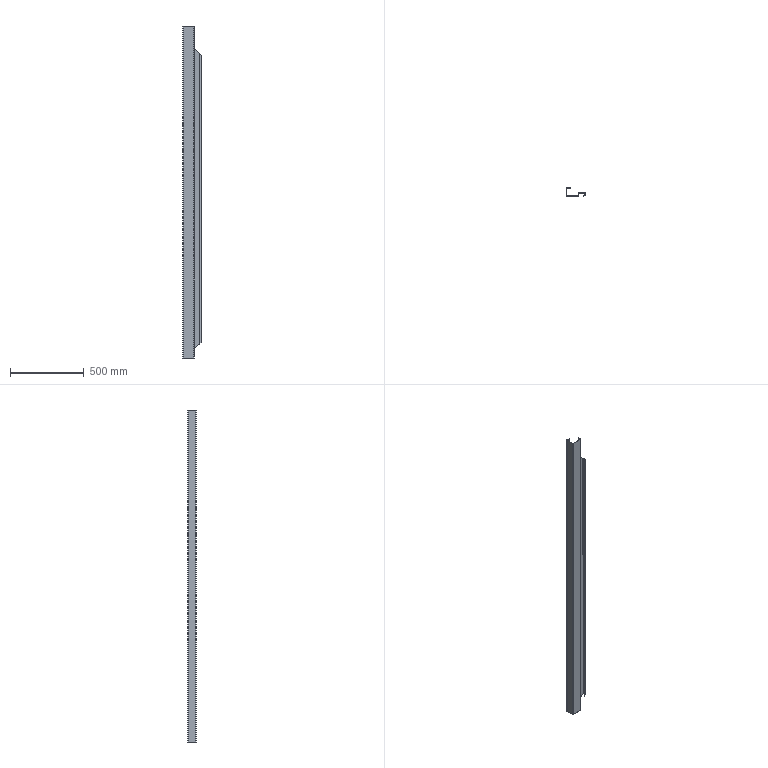Part | STEP file | 750038400 | 1 solid | 32 faces | box 127 x 60 x 2253 mm | volume 1105749 mm3 | plane 20 | cylinder 12 | commonest cylinder face diameters 4 x6 8 x6
STEP:
#1=CARTESIAN_POINT('',(4.,0.,0.));
#2=VERTEX_POINT('',#1);
#3=CARTESIAN_POINT('',(4.,0.,2252.5));
#4=VERTEX_POINT('',#3);
#5=CARTESIAN_POINT('',(4.,0.,0.));
#6=DIRECTION('',(0.,0.,1.));
#7=VECTOR('',#6,1000.);
#8=LINE('',#5,#7);
#9=EDGE_CURVE('',#2,#4,#8,.T.);
#10=ORIENTED_EDGE('',*,*,#9,.F.);
#11=CARTESIAN_POINT('',(76.,0.,0.));
#12=VERTEX_POINT('',#11);
#13=CARTESIAN_POINT('',(80.,0.,0.));
#14=DIRECTION('',(-1.,0.,0.));
#15=VECTOR('',#14,1000.);
#16=LINE('',#13,#15);
#17=EDGE_CURVE('',#12,#2,#16,.T.);
#18=ORIENTED_EDGE('',*,*,#17,.F.);
#19=CARTESIAN_POINT('',(76.,0.,2252.5));
#20=VERTEX_POINT('',#19);
#21=CARTESIAN_POINT('',(76.,0.,0.));
#22=DIRECTION('',(0.,0.,-1.));
#23=VECTOR('',#22,1000.);
#24=LINE('',#21,#23);
#25=EDGE_CURVE('',#20,#12,#24,.T.);
#26=ORIENTED_EDGE('',*,*,#25,.F.);
#27=CARTESIAN_POINT('',(80.,0.,2252.5));
#28=DIRECTION('',(1.,0.,0.));
#29=VECTOR('',#28,1000.);
#30=LINE('',#27,#29);
#31=EDGE_CURVE('',#4,#20,#30,.T.);
#32=ORIENTED_EDGE('',*,*,#31,.F.);
#33=EDGE_LOOP('',(#10,#18,#26,#32));
#34=FACE_OUTER_BOUND('',#33,.T.);
#35=CARTESIAN_POINT('',(80.,0.,0.));
#36=DIRECTION('',(0.,1.,0.));
#37=DIRECTION('',(0.,0.,1.));
#38=AXIS2_PLACEMENT_3D('',#35,#36,#37);
#39=PLANE('',#38);
#40=ADVANCED_FACE('',(#34),#39,.F.);
#41=ORIENTED_EDGE('',*,*,#31,.T.);
#42=CARTESIAN_POINT('',(80.,4.,2252.5));
#43=VERTEX_POINT('',#42);
#44=CARTESIAN_POINT('',(76.,4.,2252.5));
#45=DIRECTION('',(0.,0.,1.));
#46=DIRECTION('',(1.,0.,0.));
#47=AXIS2_PLACEMENT_3D('',#44,#45,#46);
#48=CIRCLE('',#47,4.);
#49=EDGE_CURVE('',#20,#43,#48,.T.);
#50=ORIENTED_EDGE('',*,*,#49,.T.);
#51=CARTESIAN_POINT('',(80.,26.464,2252.5));
#52=VERTEX_POINT('',#51);
#53=CARTESIAN_POINT('',(80.,10.535,2252.5));
#54=DIRECTION('',(0.,1.,0.));
#55=VECTOR('',#54,1000.);
#56=LINE('',#53,#55);
#57=EDGE_CURVE('',#43,#52,#56,.T.);
#58=ORIENTED_EDGE('',*,*,#57,.T.);
#59=CARTESIAN_POINT('',(78.,23.,2252.5));
#60=VERTEX_POINT('',#59);
#61=CARTESIAN_POINT('',(82.,23.,2252.5));
#62=DIRECTION('',(0.,0.,1.));
#63=DIRECTION('',(1.,0.,0.));
#64=AXIS2_PLACEMENT_3D('',#61,#62,#63);
#65=CIRCLE('',#64,4.);
#66=EDGE_CURVE('',#52,#60,#65,.T.);
#67=ORIENTED_EDGE('',*,*,#66,.T.);
#68=CARTESIAN_POINT('',(78.,4.,2252.5));
#69=VERTEX_POINT('',#68);
#70=CARTESIAN_POINT('',(78.,10.535,2252.5));
#71=DIRECTION('',(0.,-1.,0.));
#72=VECTOR('',#71,1000.);
#73=LINE('',#70,#72);
#74=EDGE_CURVE('',#60,#69,#73,.T.);
#75=ORIENTED_EDGE('',*,*,#74,.T.);
#76=CARTESIAN_POINT('',(76.,2.,2252.5));
#77=VERTEX_POINT('',#76);
#78=CARTESIAN_POINT('',(76.,4.,2252.5));
#79=DIRECTION('',(0.,0.,-1.));
#80=DIRECTION('',(1.,0.,0.));
#81=AXIS2_PLACEMENT_3D('',#78,#79,#80);
#82=CIRCLE('',#81,2.);
#83=EDGE_CURVE('',#69,#77,#82,.T.);
#84=ORIENTED_EDGE('',*,*,#83,.T.);
#85=CARTESIAN_POINT('',(4.,2.,2252.5));
#86=VERTEX_POINT('',#85);
#87=CARTESIAN_POINT('',(123.,2.,2252.5));
#88=DIRECTION('',(-1.,0.,0.));
#89=VECTOR('',#88,1000.);
#90=LINE('',#87,#89);
#91=EDGE_CURVE('',#77,#86,#90,.T.);
#92=ORIENTED_EDGE('',*,*,#91,.T.);
#93=CARTESIAN_POINT('',(2.,4.,2252.5));
#94=VERTEX_POINT('',#93);
#95=CARTESIAN_POINT('',(4.,4.,2252.5));
#96=DIRECTION('',(0.,0.,-1.));
#97=DIRECTION('',(1.,0.,0.));
#98=AXIS2_PLACEMENT_3D('',#95,#96,#97);
#99=CIRCLE('',#98,2.);
#100=EDGE_CURVE('',#86,#94,#99,.T.);
#101=ORIENTED_EDGE('',*,*,#100,.T.);
#102=CARTESIAN_POINT('',(2.,56.,2252.5));
#103=VERTEX_POINT('',#102);
#104=CARTESIAN_POINT('',(2.,10.535,2252.5));
#105=DIRECTION('',(0.,1.,0.));
#106=VECTOR('',#105,1000.);
#107=LINE('',#104,#106);
#108=EDGE_CURVE('',#94,#103,#107,.T.);
#109=ORIENTED_EDGE('',*,*,#108,.T.);
#110=CARTESIAN_POINT('',(4.,58.,2252.5));
#111=VERTEX_POINT('',#110);
#112=CARTESIAN_POINT('',(4.,56.,2252.5));
#113=DIRECTION('',(0.,0.,-1.));
#114=DIRECTION('',(1.,0.,0.));
#115=AXIS2_PLACEMENT_3D('',#112,#113,#114);
#116=CIRCLE('',#115,2.);
#117=EDGE_CURVE('',#103,#111,#116,.T.);
#118=ORIENTED_EDGE('',*,*,#117,.T.);
#119=CARTESIAN_POINT('',(25.,58.,2252.5));
#120=VERTEX_POINT('',#119);
#121=CARTESIAN_POINT('',(123.,58.,2252.5));
#122=DIRECTION('',(1.,0.,0.));
#123=VECTOR('',#122,1000.);
#124=LINE('',#121,#123);
#125=EDGE_CURVE('',#111,#120,#124,.T.);
#126=ORIENTED_EDGE('',*,*,#125,.T.);
#127=CARTESIAN_POINT('',(25.,60.,2252.5));
#128=VERTEX_POINT('',#127);
#129=CARTESIAN_POINT('',(25.,10.535,2252.5));
#130=DIRECTION('',(0.,1.,0.));
#131=VECTOR('',#130,1000.);
#132=LINE('',#129,#131);
#133=EDGE_CURVE('',#120,#128,#132,.T.);
#134=ORIENTED_EDGE('',*,*,#133,.T.);
#135=CARTESIAN_POINT('',(4.,60.,2252.5));
#136=VERTEX_POINT('',#135);
#137=CARTESIAN_POINT('',(123.,60.,2252.5));
#138=DIRECTION('',(-1.,0.,0.));
#139=VECTOR('',#138,1000.);
#140=LINE('',#137,#139);
#141=EDGE_CURVE('',#128,#136,#140,.T.);
#142=ORIENTED_EDGE('',*,*,#141,.T.);
#143=CARTESIAN_POINT('',(0.,56.,2252.5));
#144=VERTEX_POINT('',#143);
#145=CARTESIAN_POINT('',(4.,56.,2252.5));
#146=DIRECTION('',(0.,0.,1.));
#147=DIRECTION('',(1.,0.,0.));
#148=AXIS2_PLACEMENT_3D('',#145,#146,#147);
#149=CIRCLE('',#148,4.);
#150=EDGE_CURVE('',#136,#144,#149,.T.);
#151=ORIENTED_EDGE('',*,*,#150,.T.);
#152=CARTESIAN_POINT('',(0.,4.,2252.5));
#153=VERTEX_POINT('',#152);
#154=CARTESIAN_POINT('',(0.,10.535,2252.5));
#155=DIRECTION('',(0.,-1.,0.));
#156=VECTOR('',#155,1000.);
#157=LINE('',#154,#156);
#158=EDGE_CURVE('',#144,#153,#157,.T.);
#159=ORIENTED_EDGE('',*,*,#158,.T.);
#160=CARTESIAN_POINT('',(4.,4.,2252.5));
#161=DIRECTION('',(0.,0.,1.));
#162=DIRECTION('',(1.,0.,0.));
#163=AXIS2_PLACEMENT_3D('',#160,#161,#162);
#164=CIRCLE('',#163,4.);
#165=EDGE_CURVE('',#153,#4,#164,.T.);
#166=ORIENTED_EDGE('',*,*,#165,.T.);
#167=EDGE_LOOP('',(#41,#50,#58,#67,#75,#84,#92,#101,#109,#118,#126,#134,#142,#151,#159,#166));
#168=FACE_OUTER_BOUND('',#167,.T.);
#169=CARTESIAN_POINT('',(123.,10.535,2252.5));
#170=DIRECTION('',(0.,0.,1.));
#171=DIRECTION('',(1.,0.,0.));
#172=AXIS2_PLACEMENT_3D('',#169,#170,#171);
#173=PLANE('',#172);
#174=ADVANCED_FACE('',(#168),#173,.T.);
#175=CARTESIAN_POINT('',(0.,4.,0.));
#176=VERTEX_POINT('',#175);
#177=CARTESIAN_POINT('',(4.,4.,0.));
#178=DIRECTION('',(0.,0.,1.));
#179=DIRECTION('',(1.,0.,0.));
#180=AXIS2_PLACEMENT_3D('',#177,#178,#179);
#181=CIRCLE('',#180,4.);
#182=EDGE_CURVE('',#176,#2,#181,.T.);
#183=ORIENTED_EDGE('',*,*,#182,.T.);
#184=ORIENTED_EDGE('',*,*,#9,.T.);
#185=ORIENTED_EDGE('',*,*,#165,.F.);
#186=CARTESIAN_POINT('',(0.,4.,0.));
#187=DIRECTION('',(0.,0.,-1.));
#188=VECTOR('',#187,1000.);
#189=LINE('',#186,#188);
#190=EDGE_CURVE('',#153,#176,#189,.T.);
#191=ORIENTED_EDGE('',*,*,#190,.T.);
#192=EDGE_LOOP('',(#183,#184,#185,#191));
#193=FACE_OUTER_BOUND('',#192,.T.);
#194=CARTESIAN_POINT('',(4.,4.,0.));
#195=DIRECTION('',(0.,0.,1.));
#196=DIRECTION('',(1.,0.,0.));
#197=AXIS2_PLACEMENT_3D('',#194,#195,#196);
#198=CYLINDRICAL_SURFACE('',#197,4.);
#199=ADVANCED_FACE('',(#193),#198,.T.);
#200=CARTESIAN_POINT('',(76.,2.,0.));
#201=VERTEX_POINT('',#200);
#202=CARTESIAN_POINT('',(78.,4.,0.));
#203=VERTEX_POINT('',#202);
#204=CARTESIAN_POINT('',(76.,4.,0.));
#205=DIRECTION('',(0.,0.,1.));
#206=DIRECTION('',(1.,0.,0.));
#207=AXIS2_PLACEMENT_3D('',#204,#205,#206);
#208=CIRCLE('',#207,2.);
#209=EDGE_CURVE('',#201,#203,#208,.T.);
#210=ORIENTED_EDGE('',*,*,#209,.T.);
#211=CARTESIAN_POINT('',(78.,23.,0.));
#212=VERTEX_POINT('',#211);
#213=CARTESIAN_POINT('',(78.,6.153,0.));
#214=DIRECTION('',(0.,1.,0.));
#215=VECTOR('',#214,1000.);
#216=LINE('',#213,#215);
#217=EDGE_CURVE('',#203,#212,#216,.T.);
#218=ORIENTED_EDGE('',*,*,#217,.T.);
#219=CARTESIAN_POINT('',(80.,26.464,0.));
#220=VERTEX_POINT('',#219);
#221=CARTESIAN_POINT('',(82.,23.,0.));
#222=DIRECTION('',(0.,0.,-1.));
#223=DIRECTION('',(1.,0.,0.));
#224=AXIS2_PLACEMENT_3D('',#221,#222,#223);
#225=CIRCLE('',#224,4.);
#226=EDGE_CURVE('',#212,#220,#225,.T.);
#227=ORIENTED_EDGE('',*,*,#226,.T.);
#228=CARTESIAN_POINT('',(80.,4.,0.));
#229=VERTEX_POINT('',#228);
#230=CARTESIAN_POINT('',(80.,6.153,0.));
#231=DIRECTION('',(0.,-1.,0.));
#232=VECTOR('',#231,1000.);
#233=LINE('',#230,#232);
#234=EDGE_CURVE('',#220,#229,#233,.T.);
#235=ORIENTED_EDGE('',*,*,#234,.T.);
#236=CARTESIAN_POINT('',(76.,4.,0.));
#237=DIRECTION('',(0.,0.,-1.));
#238=DIRECTION('',(1.,0.,0.));
#239=AXIS2_PLACEMENT_3D('',#236,#237,#238);
#240=CIRCLE('',#239,4.);
#241=EDGE_CURVE('',#229,#12,#240,.T.);
#242=ORIENTED_EDGE('',*,*,#241,.T.);
#243=ORIENTED_EDGE('',*,*,#17,.T.);
#244=ORIENTED_EDGE('',*,*,#182,.F.);
#245=CARTESIAN_POINT('',(0.,56.,0.));
#246=VERTEX_POINT('',#245);
#247=CARTESIAN_POINT('',(0.,6.153,0.));
#248=DIRECTION('',(0.,1.,0.));
#249=VECTOR('',#248,1000.);
#250=LINE('',#247,#249);
#251=EDGE_CURVE('',#176,#246,#250,.T.);
#252=ORIENTED_EDGE('',*,*,#251,.T.);
#253=CARTESIAN_POINT('',(4.,60.,0.));
#254=VERTEX_POINT('',#253);
#255=CARTESIAN_POINT('',(4.,56.,0.));
#256=DIRECTION('',(0.,0.,-1.));
#257=DIRECTION('',(1.,0.,0.));
#258=AXIS2_PLACEMENT_3D('',#255,#256,#257);
#259=CIRCLE('',#258,4.);
#260=EDGE_CURVE('',#246,#254,#259,.T.);
#261=ORIENTED_EDGE('',*,*,#260,.T.);
#262=CARTESIAN_POINT('',(25.,60.,0.));
#263=VERTEX_POINT('',#262);
#264=CARTESIAN_POINT('',(114.375,60.,0.));
#265=DIRECTION('',(1.,0.,0.));
#266=VECTOR('',#265,1000.);
#267=LINE('',#264,#266);
#268=EDGE_CURVE('',#254,#263,#267,.T.);
#269=ORIENTED_EDGE('',*,*,#268,.T.);
#270=CARTESIAN_POINT('',(25.,58.,0.));
#271=VERTEX_POINT('',#270);
#272=CARTESIAN_POINT('',(25.,6.153,0.));
#273=DIRECTION('',(0.,-1.,0.));
#274=VECTOR('',#273,1000.);
#275=LINE('',#272,#274);
#276=EDGE_CURVE('',#263,#271,#275,.T.);
#277=ORIENTED_EDGE('',*,*,#276,.T.);
#278=CARTESIAN_POINT('',(4.,58.,0.));
#279=VERTEX_POINT('',#278);
#280=CARTESIAN_POINT('',(114.375,58.,0.));
#281=DIRECTION('',(-1.,0.,0.));
#282=VECTOR('',#281,1000.);
#283=LINE('',#280,#282);
#284=EDGE_CURVE('',#271,#279,#283,.T.);
#285=ORIENTED_EDGE('',*,*,#284,.T.);
#286=CARTESIAN_POINT('',(2.,56.,0.));
#287=VERTEX_POINT('',#286);
#288=CARTESIAN_POINT('',(4.,56.,0.));
#289=DIRECTION('',(0.,0.,1.));
#290=DIRECTION('',(1.,0.,0.));
#291=AXIS2_PLACEMENT_3D('',#288,#289,#290);
#292=CIRCLE('',#291,2.);
#293=EDGE_CURVE('',#279,#287,#292,.T.);
#294=ORIENTED_EDGE('',*,*,#293,.T.);
#295=CARTESIAN_POINT('',(2.,4.,0.));
#296=VERTEX_POINT('',#295);
#297=CARTESIAN_POINT('',(2.,6.153,0.));
#298=DIRECTION('',(0.,-1.,0.));
#299=VECTOR('',#298,1000.);
#300=LINE('',#297,#299);
#301=EDGE_CURVE('',#287,#296,#300,.T.);
#302=ORIENTED_EDGE('',*,*,#301,.T.);
#303=CARTESIAN_POINT('',(4.,2.,0.));
#304=VERTEX_POINT('',#303);
#305=CARTESIAN_POINT('',(4.,4.,0.));
#306=DIRECTION('',(0.,0.,1.));
#307=DIRECTION('',(1.,0.,0.));
#308=AXIS2_PLACEMENT_3D('',#305,#306,#307);
#309=CIRCLE('',#308,2.);
#310=EDGE_CURVE('',#296,#304,#309,.T.);
#311=ORIENTED_EDGE('',*,*,#310,.T.);
#312=CARTESIAN_POINT('',(114.375,2.,0.));
#313=DIRECTION('',(1.,0.,0.));
#314=VECTOR('',#313,1000.);
#315=LINE('',#312,#314);
#316=EDGE_CURVE('',#304,#201,#315,.T.);
#317=ORIENTED_EDGE('',*,*,#316,.T.);
#318=EDGE_LOOP('',(#210,#218,#227,#235,#242,#243,#244,#252,#261,#269,#277,#285,#294,#302,#311,#317));
#319=FACE_OUTER_BOUND('',#318,.T.);
#320=CARTESIAN_POINT('',(114.375,6.153,0.));
#321=DIRECTION('',(0.,0.,-1.));
#322=DIRECTION('',(-1.,0.,0.));
#323=AXIS2_PLACEMENT_3D('',#320,#321,#322);
#324=PLANE('',#323);
#325=ADVANCED_FACE('',(#319),#324,.T.);
#326=ORIENTED_EDGE('',*,*,#241,.F.);
#327=CARTESIAN_POINT('',(80.,4.,0.));
#328=DIRECTION('',(0.,0.,1.));
#329=VECTOR('',#328,1000.);
#330=LINE('',#327,#329);
#331=EDGE_CURVE('',#229,#43,#330,.T.);
#332=ORIENTED_EDGE('',*,*,#331,.T.);
#333=ORIENTED_EDGE('',*,*,#49,.F.);
#334=ORIENTED_EDGE('',*,*,#25,.T.);
#335=EDGE_LOOP('',(#326,#332,#333,#334));
#336=FACE_OUTER_BOUND('',#335,.T.);
#337=CARTESIAN_POINT('',(76.,4.,0.));
#338=DIRECTION('',(0.,0.,1.));
#339=DIRECTION('',(1.,0.,0.));
#340=AXIS2_PLACEMENT_3D('',#337,#338,#339);
#341=CYLINDRICAL_SURFACE('',#340,4.);
#342=ADVANCED_FACE('',(#336),#341,.T.);
#343=CARTESIAN_POINT('',(0.,56.,0.));
#344=DIRECTION('',(0.,0.,1.));
#345=VECTOR('',#344,1000.);
#346=LINE('',#343,#345);
#347=EDGE_CURVE('',#246,#144,#346,.T.);
#348=ORIENTED_EDGE('',*,*,#347,.F.);
#349=ORIENTED_EDGE('',*,*,#251,.F.);
#350=ORIENTED_EDGE('',*,*,#190,.F.);
#351=ORIENTED_EDGE('',*,*,#158,.F.);
#352=EDGE_LOOP('',(#348,#349,#350,#351));
#353=FACE_OUTER_BOUND('',#352,.T.);
#354=CARTESIAN_POINT('',(0.,0.,0.));
#355=DIRECTION('',(1.,0.,0.));
#356=DIRECTION('',(0.,0.,-1.));
#357=AXIS2_PLACEMENT_3D('',#354,#355,#356);
#358=PLANE('',#357);
#359=ADVANCED_FACE('',(#353),#358,.F.);
#360=ORIENTED_EDGE('',*,*,#260,.F.);
#361=ORIENTED_EDGE('',*,*,#347,.T.);
#362=ORIENTED_EDGE('',*,*,#150,.F.);
#363=CARTESIAN_POINT('',(4.,60.,0.));
#364=DIRECTION('',(0.,0.,-1.));
#365=VECTOR('',#364,1000.);
#366=LINE('',#363,#365);
#367=EDGE_CURVE('',#136,#254,#366,.T.);
#368=ORIENTED_EDGE('',*,*,#367,.T.);
#369=EDGE_LOOP('',(#360,#361,#362,#368));
#370=FACE_OUTER_BOUND('',#369,.T.);
#371=CARTESIAN_POINT('',(4.,56.,0.));
#372=DIRECTION('',(0.,0.,1.));
#373=DIRECTION('',(1.,0.,0.));
#374=AXIS2_PLACEMENT_3D('',#371,#372,#373);
#375=CYLINDRICAL_SURFACE('',#374,4.);
#376=ADVANCED_FACE('',(#370),#375,.T.);
#377=CARTESIAN_POINT('',(25.,60.,0.));
#378=DIRECTION('',(0.,0.,1.));
#379=VECTOR('',#378,1000.);
#380=LINE('',#377,#379);
#381=EDGE_CURVE('',#263,#128,#380,.T.);
#382=ORIENTED_EDGE('',*,*,#381,.F.);
#383=ORIENTED_EDGE('',*,*,#268,.F.);
#384=ORIENTED_EDGE('',*,*,#367,.F.);
#385=ORIENTED_EDGE('',*,*,#141,.F.);
#386=EDGE_LOOP('',(#382,#383,#384,#385));
#387=FACE_OUTER_BOUND('',#386,.T.);
#388=CARTESIAN_POINT('',(0.,60.,0.));
#389=DIRECTION('',(0.,-1.,0.));
#390=DIRECTION('',(0.,0.,-1.));
#391=AXIS2_PLACEMENT_3D('',#388,#389,#390);
#392=PLANE('',#391);
#393=ADVANCED_FACE('',(#387),#392,.F.);
#394=ORIENTED_EDGE('',*,*,#276,.F.);
#395=ORIENTED_EDGE('',*,*,#381,.T.);
#396=ORIENTED_EDGE('',*,*,#133,.F.);
#397=CARTESIAN_POINT('',(25.,58.,0.));
#398=DIRECTION('',(0.,0.,-1.));
#399=VECTOR('',#398,1000.);
#400=LINE('',#397,#399);
#401=EDGE_CURVE('',#120,#271,#400,.T.);
#402=ORIENTED_EDGE('',*,*,#401,.T.);
#403=EDGE_LOOP('',(#394,#395,#396,#402));
#404=FACE_OUTER_BOUND('',#403,.T.);
#405=CARTESIAN_POINT('',(25.,60.,0.));
#406=DIRECTION('',(1.,0.,0.));
#407=DIRECTION('',(0.,0.,-1.));
#408=AXIS2_PLACEMENT_3D('',#405,#406,#407);
#409=PLANE('',#408);
#410=ADVANCED_FACE('',(#404),#409,.T.);
#411=ORIENTED_EDGE('',*,*,#284,.F.);
#412=ORIENTED_EDGE('',*,*,#401,.F.);
#413=ORIENTED_EDGE('',*,*,#125,.F.);
#414=CARTESIAN_POINT('',(4.,58.,0.));
#415=DIRECTION('',(0.,0.,-1.));
#416=VECTOR('',#415,1000.);
#417=LINE('',#414,#416);
#418=EDGE_CURVE('',#111,#279,#417,.T.);
#419=ORIENTED_EDGE('',*,*,#418,.T.);
#420=EDGE_LOOP('',(#411,#412,#413,#419));
#421=FACE_OUTER_BOUND('',#420,.T.);
#422=CARTESIAN_POINT('',(0.,58.,0.));
#423=DIRECTION('',(0.,-1.,0.));
#424=DIRECTION('',(0.,0.,-1.));
#425=AXIS2_PLACEMENT_3D('',#422,#423,#424);
#426=PLANE('',#425);
#427=ADVANCED_FACE('',(#421),#426,.T.);
#428=CARTESIAN_POINT('',(2.,56.,0.));
#429=DIRECTION('',(0.,0.,1.));
#430=VECTOR('',#429,1000.);
#431=LINE('',#428,#430);
#432=EDGE_CURVE('',#287,#103,#431,.T.);
#433=ORIENTED_EDGE('',*,*,#432,.F.);
#434=ORIENTED_EDGE('',*,*,#293,.F.);
#435=ORIENTED_EDGE('',*,*,#418,.F.);
#436=ORIENTED_EDGE('',*,*,#117,.F.);
#437=EDGE_LOOP('',(#433,#434,#435,#436));
#438=FACE_OUTER_BOUND('',#437,.T.);
#439=CARTESIAN_POINT('',(4.,56.,0.));
#440=DIRECTION('',(0.,0.,1.));
#441=DIRECTION('',(1.,0.,0.));
#442=AXIS2_PLACEMENT_3D('',#439,#440,#441);
#443=CYLINDRICAL_SURFACE('',#442,2.);
#444=ADVANCED_FACE('',(#438),#443,.F.);
#445=ORIENTED_EDGE('',*,*,#301,.F.);
#446=ORIENTED_EDGE('',*,*,#432,.T.);
#447=ORIENTED_EDGE('',*,*,#108,.F.);
#448=CARTESIAN_POINT('',(2.,4.,0.));
#449=DIRECTION('',(0.,0.,-1.));
#450=VECTOR('',#449,1000.);
#451=LINE('',#448,#450);
#452=EDGE_CURVE('',#94,#296,#451,.T.);
#453=ORIENTED_EDGE('',*,*,#452,.T.);
#454=EDGE_LOOP('',(#445,#446,#447,#453));
#455=FACE_OUTER_BOUND('',#454,.T.);
#456=CARTESIAN_POINT('',(2.,0.,0.));
#457=DIRECTION('',(1.,0.,0.));
#458=DIRECTION('',(0.,0.,-1.));
#459=AXIS2_PLACEMENT_3D('',#456,#457,#458);
#460=PLANE('',#459);
#461=ADVANCED_FACE('',(#455),#460,.T.);
#462=CARTESIAN_POINT('',(4.,2.,0.));
#463=DIRECTION('',(0.,0.,1.));
#464=VECTOR('',#463,1000.);
#465=LINE('',#462,#464);
#466=EDGE_CURVE('',#304,#86,#465,.T.);
#467=ORIENTED_EDGE('',*,*,#466,.F.);
#468=ORIENTED_EDGE('',*,*,#310,.F.);
#469=ORIENTED_EDGE('',*,*,#452,.F.);
#470=ORIENTED_EDGE('',*,*,#100,.F.);
#471=EDGE_LOOP('',(#467,#468,#469,#470));
#472=FACE_OUTER_BOUND('',#471,.T.);
#473=CARTESIAN_POINT('',(4.,4.,0.));
#474=DIRECTION('',(0.,0.,1.));
#475=DIRECTION('',(1.,0.,0.));
#476=AXIS2_PLACEMENT_3D('',#473,#474,#475);
#477=CYLINDRICAL_SURFACE('',#476,2.);
#478=ADVANCED_FACE('',(#472),#477,.F.);
#479=ORIENTED_EDGE('',*,*,#316,.F.);
#480=ORIENTED_EDGE('',*,*,#466,.T.);
#481=ORIENTED_EDGE('',*,*,#91,.F.);
#482=CARTESIAN_POINT('',(76.,2.,0.));
#483=DIRECTION('',(0.,0.,-1.));
#484=VECTOR('',#483,1000.);
#485=LINE('',#482,#484);
#486=EDGE_CURVE('',#77,#201,#485,.T.);
#487=ORIENTED_EDGE('',*,*,#486,.T.);
#488=EDGE_LOOP('',(#479,#480,#481,#487));
#489=FACE_OUTER_BOUND('',#488,.T.);
#490=CARTESIAN_POINT('',(80.,2.,0.));
#491=DIRECTION('',(0.,1.,0.));
#492=DIRECTION('',(0.,0.,1.));
#493=AXIS2_PLACEMENT_3D('',#490,#491,#492);
#494=PLANE('',#493);
#495=ADVANCED_FACE('',(#489),#494,.T.);
#496=CARTESIAN_POINT('',(78.,4.,0.));
#497=DIRECTION('',(0.,0.,1.));
#498=VECTOR('',#497,1000.);
#499=LINE('',#496,#498);
#500=EDGE_CURVE('',#203,#69,#499,.T.);
#501=ORIENTED_EDGE('',*,*,#500,.F.);
#502=ORIENTED_EDGE('',*,*,#209,.F.);
#503=ORIENTED_EDGE('',*,*,#486,.F.);
#504=ORIENTED_EDGE('',*,*,#83,.F.);
#505=EDGE_LOOP('',(#501,#502,#503,#504));
#506=FACE_OUTER_BOUND('',#505,.T.);
#507=CARTESIAN_POINT('',(76.,4.,0.));
#508=DIRECTION('',(0.,0.,1.));
#509=DIRECTION('',(1.,0.,0.));
#510=AXIS2_PLACEMENT_3D('',#507,#508,#509);
#511=CYLINDRICAL_SURFACE('',#510,2.);
#512=ADVANCED_FACE('',(#506),#511,.F.);
#513=ORIENTED_EDGE('',*,*,#217,.F.);
#514=ORIENTED_EDGE('',*,*,#500,.T.);
#515=ORIENTED_EDGE('',*,*,#74,.F.);
#516=CARTESIAN_POINT('',(78.,23.,0.));
#517=DIRECTION('',(0.,0.,-1.));
#518=VECTOR('',#517,1000.);
#519=LINE('',#516,#518);
#520=EDGE_CURVE('',#60,#212,#519,.T.);
#521=ORIENTED_EDGE('',*,*,#520,.T.);
#522=EDGE_LOOP('',(#513,#514,#515,#521));
#523=FACE_OUTER_BOUND('',#522,.T.);
#524=CARTESIAN_POINT('',(78.,25.,0.));
#525=DIRECTION('',(-1.,0.,0.));
#526=DIRECTION('',(0.,-1.,0.));
#527=AXIS2_PLACEMENT_3D('',#524,#525,#526);
#528=PLANE('',#527);
#529=ADVANCED_FACE('',(#523),#528,.T.);
#530=CARTESIAN_POINT('',(82.,27.,2098.));
#531=VERTEX_POINT('',#530);
#532=CARTESIAN_POINT('',(82.,27.,62.));
#533=VERTEX_POINT('',#532);
#534=CARTESIAN_POINT('',(82.,27.,0.));
#535=DIRECTION('',(0.,0.,-1.));
#536=VECTOR('',#535,1000.);
#537=LINE('',#534,#536);
#538=EDGE_CURVE('',#531,#533,#537,.T.);
#539=ORIENTED_EDGE('',*,*,#538,.T.);
#540=CARTESIAN_POINT('',(80.,26.464,60.));
#541=VERTEX_POINT('',#540);
#542=CARTESIAN_POINT('',(82.,27.,62.));
#543=CARTESIAN_POINT('',(81.294,27.,61.294));
#544=CARTESIAN_POINT('',(80.612,26.817,60.612));
#545=CARTESIAN_POINT('',(80.,26.464,60.));
#546=(BOUNDED_CURVE()B_SPLINE_CURVE(3,(#542,#543,#544,#545),.UNSPECIFIED.,.F.,.F.)B_SPLINE_CURVE_WITH_KNOTS((4,4),(1.571,2.094),.UNSPECIFIED.)CURVE()GEOMETRIC_REPRESENTATION_ITEM()RATIONAL_B_SPLINE_CURVE((1.,0.9773,0.9773,1.))REPRESENTATION_ITEM(''));
#547=EDGE_CURVE('',#533,#541,#546,.T.);
#548=ORIENTED_EDGE('',*,*,#547,.T.);
#549=CARTESIAN_POINT('',(80.,26.464,0.));
#550=DIRECTION('',(0.,0.,-1.));
#551=VECTOR('',#550,1000.);
#552=LINE('',#549,#551);
#553=EDGE_CURVE('',#541,#220,#552,.T.);
#554=ORIENTED_EDGE('',*,*,#553,.T.);
#555=ORIENTED_EDGE('',*,*,#226,.F.);
#556=ORIENTED_EDGE('',*,*,#520,.F.);
#557=ORIENTED_EDGE('',*,*,#66,.F.);
#558=CARTESIAN_POINT('',(80.,26.464,2100.));
#559=VERTEX_POINT('',#558);
#560=CARTESIAN_POINT('',(80.,26.464,0.));
#561=DIRECTION('',(0.,0.,-1.));
#562=VECTOR('',#561,1000.);
#563=LINE('',#560,#562);
#564=EDGE_CURVE('',#52,#559,#563,.T.);
#565=ORIENTED_EDGE('',*,*,#564,.T.);
#566=CARTESIAN_POINT('',(80.,26.464,2100.));
#567=CARTESIAN_POINT('',(80.612,26.817,2099.388));
#568=CARTESIAN_POINT('',(81.294,27.,2098.706));
#569=CARTESIAN_POINT('',(82.,27.,2098.));
#570=(BOUNDED_CURVE()B_SPLINE_CURVE(3,(#566,#567,#568,#569),.UNSPECIFIED.,.F.,.F.)B_SPLINE_CURVE_WITH_KNOTS((4,4),(1.047,1.571),.UNSPECIFIED.)CURVE()GEOMETRIC_REPRESENTATION_ITEM()RATIONAL_B_SPLINE_CURVE((1.,0.9773,0.9773,1.))REPRESENTATION_ITEM(''));
#571=EDGE_CURVE('',#559,#531,#570,.T.);
#572=ORIENTED_EDGE('',*,*,#571,.T.);
#573=EDGE_LOOP('',(#539,#548,#554,#555,#556,#557,#565,#572));
#574=FACE_OUTER_BOUND('',#573,.T.);
#575=CARTESIAN_POINT('',(82.,23.,0.));
#576=DIRECTION('',(0.,0.,1.));
#577=DIRECTION('',(1.,0.,0.));
#578=AXIS2_PLACEMENT_3D('',#575,#576,#577);
#579=CYLINDRICAL_SURFACE('',#578,4.);
#580=ADVANCED_FACE('',(#574),#579,.T.);
#581=ORIENTED_EDGE('',*,*,#553,.F.);
#582=CARTESIAN_POINT('',(80.,23.,60.));
#583=VERTEX_POINT('',#582);
#584=CARTESIAN_POINT('',(80.,25.,60.));
#585=DIRECTION('',(0.,1.,0.));
#586=VECTOR('',#585,1000.);
#587=LINE('',#584,#586);
#588=EDGE_CURVE('',#583,#541,#587,.T.);
#589=ORIENTED_EDGE('',*,*,#588,.F.);
#590=CARTESIAN_POINT('',(80.,23.,2100.));
#591=VERTEX_POINT('',#590);
#592=CARTESIAN_POINT('',(80.,23.,0.));
#593=DIRECTION('',(0.,0.,-1.));
#594=VECTOR('',#593,1000.);
#595=LINE('',#592,#594);
#596=EDGE_CURVE('',#591,#583,#595,.T.);
#597=ORIENTED_EDGE('',*,*,#596,.F.);
#598=CARTESIAN_POINT('',(80.,25.,2100.));
#599=DIRECTION('',(0.,-1.,0.));
#600=VECTOR('',#599,1000.);
#601=LINE('',#598,#600);
#602=EDGE_CURVE('',#559,#591,#601,.T.);
#603=ORIENTED_EDGE('',*,*,#602,.F.);
#604=ORIENTED_EDGE('',*,*,#564,.F.);
#605=ORIENTED_EDGE('',*,*,#57,.F.);
#606=ORIENTED_EDGE('',*,*,#331,.F.);
#607=ORIENTED_EDGE('',*,*,#234,.F.);
#608=EDGE_LOOP('',(#581,#589,#597,#603,#604,#605,#606,#607));
#609=FACE_OUTER_BOUND('',#608,.T.);
#610=CARTESIAN_POINT('',(80.,25.,0.));
#611=DIRECTION('',(-1.,0.,0.));
#612=DIRECTION('',(0.,-1.,0.));
#613=AXIS2_PLACEMENT_3D('',#610,#611,#612);
#614=PLANE('',#613);
#615=ADVANCED_FACE('',(#609),#614,.F.);
#616=ORIENTED_EDGE('',*,*,#547,.F.);
#617=CARTESIAN_POINT('',(123.,27.,103.));
#618=VERTEX_POINT('',#617);
#619=CARTESIAN_POINT('',(127.376,27.,107.376));
#620=DIRECTION('',(-0.7071,0.,-0.7071));
#621=VECTOR('',#620,1000.);
#622=LINE('',#619,#621);
#623=EDGE_CURVE('',#618,#533,#622,.T.);
#624=ORIENTED_EDGE('',*,*,#623,.F.);
#625=CARTESIAN_POINT('',(127.,23.,107.));
#626=VERTEX_POINT('',#625);
#627=CARTESIAN_POINT('',(127.,23.,107.));
#628=CARTESIAN_POINT('',(127.,25.343,107.));
#629=CARTESIAN_POINT('',(125.343,27.,105.343));
#630=CARTESIAN_POINT('',(123.,27.,103.));
#631=(BOUNDED_CURVE()B_SPLINE_CURVE(3,(#627,#628,#629,#630),.UNSPECIFIED.,.F.,.F.)B_SPLINE_CURVE_WITH_KNOTS((4,4),(0.,1.571),.UNSPECIFIED.)CURVE()GEOMETRIC_REPRESENTATION_ITEM()RATIONAL_B_SPLINE_CURVE((1.,0.8047,0.8047,1.))REPRESENTATION_ITEM(''));
#632=EDGE_CURVE('',#626,#618,#631,.T.);
#633=ORIENTED_EDGE('',*,*,#632,.F.);
#634=CARTESIAN_POINT('',(127.,10.535,107.));
#635=VERTEX_POINT('',#634);
#636=CARTESIAN_POINT('',(127.,66.,107.));
#637=DIRECTION('',(0.,1.,0.));
#638=VECTOR('',#637,1000.);
#639=LINE('',#636,#638);
#640=EDGE_CURVE('',#635,#626,#639,.T.);
#641=ORIENTED_EDGE('',*,*,#640,.F.);
#642=CARTESIAN_POINT('',(124.035,6.671,104.035));
#643=VERTEX_POINT('',#642);
#644=CARTESIAN_POINT('',(124.035,6.671,104.035));
#645=CARTESIAN_POINT('',(125.854,7.158,105.854));
#646=CARTESIAN_POINT('',(127.,8.652,107.));
#647=CARTESIAN_POINT('',(127.,10.535,107.));
#648=(BOUNDED_CURVE()B_SPLINE_CURVE(3,(#644,#645,#646,#647),.UNSPECIFIED.,.F.,.F.)B_SPLINE_CURVE_WITH_KNOTS((4,4),(4.974,6.283),.UNSPECIFIED.)CURVE()GEOMETRIC_REPRESENTATION_ITEM()RATIONAL_B_SPLINE_CURVE((1.,0.8622,0.8622,1.))REPRESENTATION_ITEM(''));
#649=EDGE_CURVE('',#643,#635,#648,.T.);
#650=ORIENTED_EDGE('',*,*,#649,.F.);
#651=CARTESIAN_POINT('',(114.892,4.221,94.892));
#652=VERTEX_POINT('',#651);
#653=CARTESIAN_POINT('',(114.892,4.221,94.892));
#654=DIRECTION('',(0.6947,0.1862,0.6947));
#655=VECTOR('',#654,1000.);
#656=LINE('',#653,#655);
#657=EDGE_CURVE('',#652,#643,#656,.T.);
#658=ORIENTED_EDGE('',*,*,#657,.F.);
#659=CARTESIAN_POINT('',(114.375,6.153,94.375));
#660=VERTEX_POINT('',#659);
#661=CARTESIAN_POINT('',(114.375,6.153,94.375));
#662=DIRECTION('',(0.2506,-0.9351,0.2506));
#663=VECTOR('',#662,1000.);
#664=LINE('',#661,#663);
#665=EDGE_CURVE('',#660,#652,#664,.T.);
#666=ORIENTED_EDGE('',*,*,#665,.F.);
#667=CARTESIAN_POINT('',(123.518,8.603,103.518));
#668=VERTEX_POINT('',#667);
#669=CARTESIAN_POINT('',(123.518,8.603,103.518));
#670=DIRECTION('',(-0.6947,-0.1862,-0.6947));
#671=VECTOR('',#670,1000.);
#672=LINE('',#669,#671);
#673=EDGE_CURVE('',#668,#660,#672,.T.);
#674=ORIENTED_EDGE('',*,*,#673,.F.);
#675=CARTESIAN_POINT('',(125.,10.535,105.));
#676=VERTEX_POINT('',#675);
#677=CARTESIAN_POINT('',(125.,10.535,105.));
#678=CARTESIAN_POINT('',(125.,9.593,105.));
#679=CARTESIAN_POINT('',(124.427,8.846,104.427));
#680=CARTESIAN_POINT('',(123.518,8.603,103.518));
#681=(BOUNDED_CURVE()B_SPLINE_CURVE(3,(#677,#678,#679,#680),.UNSPECIFIED.,.F.,.F.)B_SPLINE_CURVE_WITH_KNOTS((4,4),(0.,1.309),.UNSPECIFIED.)CURVE()GEOMETRIC_REPRESENTATION_ITEM()RATIONAL_B_SPLINE_CURVE((1.,0.8622,0.8622,1.))REPRESENTATION_ITEM(''));
#682=EDGE_CURVE('',#676,#668,#681,.T.);
#683=ORIENTED_EDGE('',*,*,#682,.F.);
#684=CARTESIAN_POINT('',(125.,23.,105.));
#685=VERTEX_POINT('',#684);
#686=CARTESIAN_POINT('',(125.,66.,105.));
#687=DIRECTION('',(0.,-1.,0.));
#688=VECTOR('',#687,1000.);
#689=LINE('',#686,#688);
#690=EDGE_CURVE('',#685,#676,#689,.T.);
#691=ORIENTED_EDGE('',*,*,#690,.F.);
#692=CARTESIAN_POINT('',(123.,25.,103.));
#693=VERTEX_POINT('',#692);
#694=CARTESIAN_POINT('',(123.,25.,103.));
#695=CARTESIAN_POINT('',(124.172,25.,104.172));
#696=CARTESIAN_POINT('',(125.,24.172,105.));
#697=CARTESIAN_POINT('',(125.,23.,105.));
#698=(BOUNDED_CURVE()B_SPLINE_CURVE(3,(#694,#695,#696,#697),.UNSPECIFIED.,.F.,.F.)B_SPLINE_CURVE_WITH_KNOTS((4,4),(4.712,6.283),.UNSPECIFIED.)CURVE()GEOMETRIC_REPRESENTATION_ITEM()RATIONAL_B_SPLINE_CURVE((1.,0.8047,0.8047,1.))REPRESENTATION_ITEM(''));
#699=EDGE_CURVE('',#693,#685,#698,.T.);
#700=ORIENTED_EDGE('',*,*,#699,.F.);
#701=CARTESIAN_POINT('',(82.,25.,62.));
#702=VERTEX_POINT('',#701);
#703=CARTESIAN_POINT('',(127.376,25.,107.376));
#704=DIRECTION('',(0.7071,0.,0.7071));
#705=VECTOR('',#704,1000.);
#706=LINE('',#703,#705);
#707=EDGE_CURVE('',#702,#693,#706,.T.);
#708=ORIENTED_EDGE('',*,*,#707,.F.);
#709=CARTESIAN_POINT('',(80.,23.,60.));
#710=CARTESIAN_POINT('',(80.,24.172,60.));
#711=CARTESIAN_POINT('',(80.828,25.,60.828));
#712=CARTESIAN_POINT('',(82.,25.,62.));
#713=(BOUNDED_CURVE()B_SPLINE_CURVE(3,(#709,#710,#711,#712),.UNSPECIFIED.,.F.,.F.)B_SPLINE_CURVE_WITH_KNOTS((4,4),(3.142,4.712),.UNSPECIFIED.)CURVE()GEOMETRIC_REPRESENTATION_ITEM()RATIONAL_B_SPLINE_CURVE((1.,0.8047,0.8047,1.))REPRESENTATION_ITEM(''));
#714=EDGE_CURVE('',#583,#702,#713,.T.);
#715=ORIENTED_EDGE('',*,*,#714,.F.);
#716=ORIENTED_EDGE('',*,*,#588,.T.);
#717=EDGE_LOOP('',(#616,#624,#633,#641,#650,#658,#666,#674,#683,#691,#700,#708,#715,#716));
#718=FACE_OUTER_BOUND('',#717,.T.);
#719=CARTESIAN_POINT('',(127.376,66.,107.376));
#720=DIRECTION('',(-0.7071,0.,0.7071));
#721=DIRECTION('',(0.7071,0.,0.7071));
#722=AXIS2_PLACEMENT_3D('',#719,#720,#721);
#723=PLANE('',#722);
#724=ADVANCED_FACE('',(#718),#723,.F.);
#725=CARTESIAN_POINT('',(123.,27.,2057.));
#726=VERTEX_POINT('',#725);
#727=CARTESIAN_POINT('',(82.,27.,2098.));
#728=DIRECTION('',(0.7071,0.,-0.7071));
#729=VECTOR('',#728,1000.);
#730=LINE('',#727,#729);
#731=EDGE_CURVE('',#531,#726,#730,.T.);
#732=ORIENTED_EDGE('',*,*,#731,.T.);
#733=CARTESIAN_POINT('',(123.,27.,0.));
#734=DIRECTION('',(0.,0.,-1.));
#735=VECTOR('',#734,1000.);
#736=LINE('',#733,#735);
#737=EDGE_CURVE('',#726,#618,#736,.T.);
#738=ORIENTED_EDGE('',*,*,#737,.T.);
#739=ORIENTED_EDGE('',*,*,#623,.T.);
#740=ORIENTED_EDGE('',*,*,#538,.F.);
#741=EDGE_LOOP('',(#732,#738,#739,#740));
#742=FACE_OUTER_BOUND('',#741,.T.);
#743=CARTESIAN_POINT('',(125.,27.,0.));
#744=DIRECTION('',(0.,1.,0.));
#745=DIRECTION('',(0.,0.,1.));
#746=AXIS2_PLACEMENT_3D('',#743,#744,#745);
#747=PLANE('',#746);
#748=ADVANCED_FACE('',(#742),#747,.T.);
#749=CARTESIAN_POINT('',(125.,23.,2055.));
#750=VERTEX_POINT('',#749);
#751=CARTESIAN_POINT('',(123.,25.,2057.));
#752=VERTEX_POINT('',#751);
#753=CARTESIAN_POINT('',(125.,23.,2055.));
#754=CARTESIAN_POINT('',(125.,24.172,2055.));
#755=CARTESIAN_POINT('',(124.172,25.,2055.828));
#756=CARTESIAN_POINT('',(123.,25.,2057.));
#757=(BOUNDED_CURVE()B_SPLINE_CURVE(3,(#753,#754,#755,#756),.UNSPECIFIED.,.F.,.T.)B_SPLINE_CURVE_WITH_KNOTS((4,4),(3.142,4.712),.UNSPECIFIED.)CURVE()GEOMETRIC_REPRESENTATION_ITEM()RATIONAL_B_SPLINE_CURVE((1.,0.8047,0.8047,1.))REPRESENTATION_ITEM(''));
#758=EDGE_CURVE('',#750,#752,#757,.T.);
#759=ORIENTED_EDGE('',*,*,#758,.F.);
#760=CARTESIAN_POINT('',(125.,10.535,2055.));
#761=VERTEX_POINT('',#760);
#762=CARTESIAN_POINT('',(125.,66.,2055.));
#763=DIRECTION('',(0.,1.,0.));
#764=VECTOR('',#763,1000.);
#765=LINE('',#762,#764);
#766=EDGE_CURVE('',#761,#750,#765,.T.);
#767=ORIENTED_EDGE('',*,*,#766,.F.);
#768=CARTESIAN_POINT('',(123.518,8.603,2056.482));
#769=VERTEX_POINT('',#768);
#770=CARTESIAN_POINT('',(123.518,8.603,2056.482));
#771=CARTESIAN_POINT('',(124.427,8.846,2055.573));
#772=CARTESIAN_POINT('',(125.,9.593,2055.));
#773=CARTESIAN_POINT('',(125.,10.535,2055.));
#774=(BOUNDED_CURVE()B_SPLINE_CURVE(3,(#770,#771,#772,#773),.UNSPECIFIED.,.F.,.F.)B_SPLINE_CURVE_WITH_KNOTS((4,4),(1.833,3.142),.UNSPECIFIED.)CURVE()GEOMETRIC_REPRESENTATION_ITEM()RATIONAL_B_SPLINE_CURVE((1.,0.8622,0.8622,1.))REPRESENTATION_ITEM(''));
#775=EDGE_CURVE('',#769,#761,#774,.T.);
#776=ORIENTED_EDGE('',*,*,#775,.F.);
#777=CARTESIAN_POINT('',(114.375,6.153,2065.625));
#778=VERTEX_POINT('',#777);
#779=CARTESIAN_POINT('',(114.375,6.153,2065.625));
#780=DIRECTION('',(0.6947,0.1862,-0.6947));
#781=VECTOR('',#780,1000.);
#782=LINE('',#779,#781);
#783=EDGE_CURVE('',#778,#769,#782,.T.);
#784=ORIENTED_EDGE('',*,*,#783,.F.);
#785=CARTESIAN_POINT('',(114.892,4.221,2065.108));
#786=VERTEX_POINT('',#785);
#787=CARTESIAN_POINT('',(114.892,4.221,2065.108));
#788=DIRECTION('',(-0.2506,0.9351,0.2506));
#789=VECTOR('',#788,1000.);
#790=LINE('',#787,#789);
#791=EDGE_CURVE('',#786,#778,#790,.T.);
#792=ORIENTED_EDGE('',*,*,#791,.F.);
#793=CARTESIAN_POINT('',(124.035,6.671,2055.965));
#794=VERTEX_POINT('',#793);
#795=CARTESIAN_POINT('',(124.035,6.671,2055.965));
#796=DIRECTION('',(-0.6947,-0.1862,0.6947));
#797=VECTOR('',#796,1000.);
#798=LINE('',#795,#797);
#799=EDGE_CURVE('',#794,#786,#798,.T.);
#800=ORIENTED_EDGE('',*,*,#799,.F.);
#801=CARTESIAN_POINT('',(127.,10.535,2053.));
#802=VERTEX_POINT('',#801);
#803=CARTESIAN_POINT('',(127.,10.535,2053.));
#804=CARTESIAN_POINT('',(127.,8.652,2053.));
#805=CARTESIAN_POINT('',(125.854,7.158,2054.146));
#806=CARTESIAN_POINT('',(124.035,6.671,2055.965));
#807=(BOUNDED_CURVE()B_SPLINE_CURVE(3,(#803,#804,#805,#806),.UNSPECIFIED.,.F.,.F.)B_SPLINE_CURVE_WITH_KNOTS((4,4),(3.142,4.451),.UNSPECIFIED.)CURVE()GEOMETRIC_REPRESENTATION_ITEM()RATIONAL_B_SPLINE_CURVE((1.,0.8622,0.8622,1.))REPRESENTATION_ITEM(''));
#808=EDGE_CURVE('',#802,#794,#807,.T.);
#809=ORIENTED_EDGE('',*,*,#808,.F.);
#810=CARTESIAN_POINT('',(127.,23.,2053.));
#811=VERTEX_POINT('',#810);
#812=CARTESIAN_POINT('',(127.,66.,2053.));
#813=DIRECTION('',(0.,-1.,0.));
#814=VECTOR('',#813,1000.);
#815=LINE('',#812,#814);
#816=EDGE_CURVE('',#811,#802,#815,.T.);
#817=ORIENTED_EDGE('',*,*,#816,.F.);
#818=CARTESIAN_POINT('',(123.,27.,2057.));
#819=CARTESIAN_POINT('',(125.343,27.,2054.657));
#820=CARTESIAN_POINT('',(127.,25.343,2053.));
#821=CARTESIAN_POINT('',(127.,23.,2053.));
#822=(BOUNDED_CURVE()B_SPLINE_CURVE(3,(#818,#819,#820,#821),.UNSPECIFIED.,.F.,.F.)B_SPLINE_CURVE_WITH_KNOTS((4,4),(1.571,3.142),.UNSPECIFIED.)CURVE()GEOMETRIC_REPRESENTATION_ITEM()RATIONAL_B_SPLINE_CURVE((1.,0.8047,0.8047,1.))REPRESENTATION_ITEM(''));
#823=EDGE_CURVE('',#726,#811,#822,.T.);
#824=ORIENTED_EDGE('',*,*,#823,.F.);
#825=ORIENTED_EDGE('',*,*,#731,.F.);
#826=ORIENTED_EDGE('',*,*,#571,.F.);
#827=ORIENTED_EDGE('',*,*,#602,.T.);
#828=CARTESIAN_POINT('',(82.,25.,2098.));
#829=VERTEX_POINT('',#828);
#830=CARTESIAN_POINT('',(82.,25.,2098.));
#831=CARTESIAN_POINT('',(80.828,25.,2099.172));
#832=CARTESIAN_POINT('',(80.,24.172,2100.));
#833=CARTESIAN_POINT('',(80.,23.,2100.));
#834=(BOUNDED_CURVE()B_SPLINE_CURVE(3,(#830,#831,#832,#833),.UNSPECIFIED.,.F.,.T.)B_SPLINE_CURVE_WITH_KNOTS((4,4),(4.712,6.283),.UNSPECIFIED.)CURVE()GEOMETRIC_REPRESENTATION_ITEM()RATIONAL_B_SPLINE_CURVE((1.,0.8047,0.8047,1.))REPRESENTATION_ITEM(''));
#835=EDGE_CURVE('',#829,#591,#834,.T.);
#836=ORIENTED_EDGE('',*,*,#835,.F.);
#837=CARTESIAN_POINT('',(80.,25.,2100.));
#838=DIRECTION('',(-0.7071,0.,0.7071));
#839=VECTOR('',#838,1000.);
#840=LINE('',#837,#839);
#841=EDGE_CURVE('',#752,#829,#840,.T.);
#842=ORIENTED_EDGE('',*,*,#841,.F.);
#843=EDGE_LOOP('',(#759,#767,#776,#784,#792,#800,#809,#817,#824,#825,#826,#827,#836,#842));
#844=FACE_OUTER_BOUND('',#843,.T.);
#845=CARTESIAN_POINT('',(80.,66.,2100.));
#846=DIRECTION('',(-0.7071,0.,-0.7071));
#847=DIRECTION('',(-0.7071,0.,0.7071));
#848=AXIS2_PLACEMENT_3D('',#845,#846,#847);
#849=PLANE('',#848);
#850=ADVANCED_FACE('',(#844),#849,.F.);
#851=ORIENTED_EDGE('',*,*,#714,.T.);
#852=CARTESIAN_POINT('',(82.,25.,0.));
#853=DIRECTION('',(0.,0.,-1.));
#854=VECTOR('',#853,1000.);
#855=LINE('',#852,#854);
#856=EDGE_CURVE('',#829,#702,#855,.T.);
#857=ORIENTED_EDGE('',*,*,#856,.F.);
#858=ORIENTED_EDGE('',*,*,#835,.T.);
#859=ORIENTED_EDGE('',*,*,#596,.T.);
#860=EDGE_LOOP('',(#851,#857,#858,#859));
#861=FACE_OUTER_BOUND('',#860,.T.);
#862=CARTESIAN_POINT('',(82.,23.,0.));
#863=DIRECTION('',(0.,0.,1.));
#864=DIRECTION('',(1.,0.,0.));
#865=AXIS2_PLACEMENT_3D('',#862,#863,#864);
#866=CYLINDRICAL_SURFACE('',#865,2.);
#867=ADVANCED_FACE('',(#861),#866,.F.);
#868=ORIENTED_EDGE('',*,*,#823,.T.);
#869=CARTESIAN_POINT('',(127.,23.,0.));
#870=DIRECTION('',(0.,0.,-1.));
#871=VECTOR('',#870,1000.);
#872=LINE('',#869,#871);
#873=EDGE_CURVE('',#811,#626,#872,.T.);
#874=ORIENTED_EDGE('',*,*,#873,.T.);
#875=ORIENTED_EDGE('',*,*,#632,.T.);
#876=ORIENTED_EDGE('',*,*,#737,.F.);
#877=EDGE_LOOP('',(#868,#874,#875,#876));
#878=FACE_OUTER_BOUND('',#877,.T.);
#879=CARTESIAN_POINT('',(123.,23.,0.));
#880=DIRECTION('',(0.,0.,1.));
#881=DIRECTION('',(1.,0.,0.));
#882=AXIS2_PLACEMENT_3D('',#879,#880,#881);
#883=CYLINDRICAL_SURFACE('',#882,4.);
#884=ADVANCED_FACE('',(#878),#883,.T.);
#885=CARTESIAN_POINT('',(127.,10.535,0.));
#886=DIRECTION('',(0.,0.,-1.));
#887=VECTOR('',#886,1000.);
#888=LINE('',#885,#887);
#889=EDGE_CURVE('',#802,#635,#888,.T.);
#890=ORIENTED_EDGE('',*,*,#889,.T.);
#891=ORIENTED_EDGE('',*,*,#640,.T.);
#892=ORIENTED_EDGE('',*,*,#873,.F.);
#893=ORIENTED_EDGE('',*,*,#816,.T.);
#894=EDGE_LOOP('',(#890,#891,#892,#893));
#895=FACE_OUTER_BOUND('',#894,.T.);
#896=CARTESIAN_POINT('',(127.,9.,0.));
#897=DIRECTION('',(1.,0.,0.));
#898=DIRECTION('',(0.,1.,0.));
#899=AXIS2_PLACEMENT_3D('',#896,#897,#898);
#900=PLANE('',#899);
#901=ADVANCED_FACE('',(#895),#900,.T.);
#902=ORIENTED_EDGE('',*,*,#808,.T.);
#903=CARTESIAN_POINT('',(124.035,6.671,0.));
#904=DIRECTION('',(0.,0.,-1.));
#905=VECTOR('',#904,1000.);
#906=LINE('',#903,#905);
#907=EDGE_CURVE('',#794,#643,#906,.T.);
#908=ORIENTED_EDGE('',*,*,#907,.T.);
#909=ORIENTED_EDGE('',*,*,#649,.T.);
#910=ORIENTED_EDGE('',*,*,#889,.F.);
#911=EDGE_LOOP('',(#902,#908,#909,#910));
#912=FACE_OUTER_BOUND('',#911,.T.);
#913=CARTESIAN_POINT('',(123.,10.535,0.));
#914=DIRECTION('',(0.,0.,1.));
#915=DIRECTION('',(1.,0.,0.));
#916=AXIS2_PLACEMENT_3D('',#913,#914,#915);
#917=CYLINDRICAL_SURFACE('',#916,4.);
#918=ADVANCED_FACE('',(#912),#917,.T.);
#919=ORIENTED_EDGE('',*,*,#799,.T.);
#920=CARTESIAN_POINT('',(114.892,4.221,0.));
#921=DIRECTION('',(0.,0.,-1.));
#922=VECTOR('',#921,1000.);
#923=LINE('',#920,#922);
#924=EDGE_CURVE('',#786,#652,#923,.T.);
#925=ORIENTED_EDGE('',*,*,#924,.T.);
#926=ORIENTED_EDGE('',*,*,#657,.T.);
#927=ORIENTED_EDGE('',*,*,#907,.F.);
#928=EDGE_LOOP('',(#919,#925,#926,#927));
#929=FACE_OUTER_BOUND('',#928,.T.);
#930=CARTESIAN_POINT('',(114.892,4.221,0.));
#931=DIRECTION('',(0.2588,-0.9659,0.));
#932=DIRECTION('',(0.9659,0.2588,0.));
#933=AXIS2_PLACEMENT_3D('',#930,#931,#932);
#934=PLANE('',#933);
#935=ADVANCED_FACE('',(#929),#934,.T.);
#936=ORIENTED_EDGE('',*,*,#924,.F.);
#937=ORIENTED_EDGE('',*,*,#791,.T.);
#938=CARTESIAN_POINT('',(114.375,6.153,0.));
#939=DIRECTION('',(0.,0.,1.));
#940=VECTOR('',#939,1000.);
#941=LINE('',#938,#940);
#942=EDGE_CURVE('',#660,#778,#941,.T.);
#943=ORIENTED_EDGE('',*,*,#942,.F.);
#944=ORIENTED_EDGE('',*,*,#665,.T.);
#945=EDGE_LOOP('',(#936,#937,#943,#944));
#946=FACE_OUTER_BOUND('',#945,.T.);
#947=CARTESIAN_POINT('',(114.375,6.153,0.));
#948=DIRECTION('',(0.9659,0.2588,0.));
#949=DIRECTION('',(-0.2588,0.9659,0.));
#950=AXIS2_PLACEMENT_3D('',#947,#948,#949);
#951=PLANE('',#950);
#952=ADVANCED_FACE('',(#946),#951,.F.);
#953=ORIENTED_EDGE('',*,*,#673,.T.);
#954=ORIENTED_EDGE('',*,*,#942,.T.);
#955=ORIENTED_EDGE('',*,*,#783,.T.);
#956=CARTESIAN_POINT('',(123.518,8.603,0.));
#957=DIRECTION('',(0.,0.,1.));
#958=VECTOR('',#957,1000.);
#959=LINE('',#956,#958);
#960=EDGE_CURVE('',#668,#769,#959,.T.);
#961=ORIENTED_EDGE('',*,*,#960,.F.);
#962=EDGE_LOOP('',(#953,#954,#955,#961));
#963=FACE_OUTER_BOUND('',#962,.T.);
#964=CARTESIAN_POINT('',(114.375,6.153,0.));
#965=DIRECTION('',(0.2588,-0.9659,0.));
#966=DIRECTION('',(0.9659,0.2588,0.));
#967=AXIS2_PLACEMENT_3D('',#964,#965,#966);
#968=PLANE('',#967);
#969=ADVANCED_FACE('',(#963),#968,.F.);
#970=ORIENTED_EDGE('',*,*,#682,.T.);
#971=ORIENTED_EDGE('',*,*,#960,.T.);
#972=ORIENTED_EDGE('',*,*,#775,.T.);
#973=CARTESIAN_POINT('',(125.,10.535,0.));
#974=DIRECTION('',(0.,0.,1.));
#975=VECTOR('',#974,1000.);
#976=LINE('',#973,#975);
#977=EDGE_CURVE('',#676,#761,#976,.T.);
#978=ORIENTED_EDGE('',*,*,#977,.F.);
#979=EDGE_LOOP('',(#970,#971,#972,#978));
#980=FACE_OUTER_BOUND('',#979,.T.);
#981=CARTESIAN_POINT('',(123.,10.535,0.));
#982=DIRECTION('',(0.,0.,1.));
#983=DIRECTION('',(1.,0.,0.));
#984=AXIS2_PLACEMENT_3D('',#981,#982,#983);
#985=CYLINDRICAL_SURFACE('',#984,2.);
#986=ADVANCED_FACE('',(#980),#985,.F.);
#987=ORIENTED_EDGE('',*,*,#690,.T.);
#988=ORIENTED_EDGE('',*,*,#977,.T.);
#989=ORIENTED_EDGE('',*,*,#766,.T.);
#990=CARTESIAN_POINT('',(125.,23.,0.));
#991=DIRECTION('',(0.,0.,1.));
#992=VECTOR('',#991,1000.);
#993=LINE('',#990,#992);
#994=EDGE_CURVE('',#685,#750,#993,.T.);
#995=ORIENTED_EDGE('',*,*,#994,.F.);
#996=EDGE_LOOP('',(#987,#988,#989,#995));
#997=FACE_OUTER_BOUND('',#996,.T.);
#998=CARTESIAN_POINT('',(125.,9.,0.));
#999=DIRECTION('',(1.,0.,0.));
#1000=DIRECTION('',(0.,1.,0.));
#1001=AXIS2_PLACEMENT_3D('',#998,#999,#1000);
#1002=PLANE('',#1001);
#1003=ADVANCED_FACE('',(#997),#1002,.F.);
#1004=ORIENTED_EDGE('',*,*,#699,.T.);
#1005=ORIENTED_EDGE('',*,*,#994,.T.);
#1006=ORIENTED_EDGE('',*,*,#758,.T.);
#1007=CARTESIAN_POINT('',(123.,25.,0.));
#1008=DIRECTION('',(0.,0.,1.));
#1009=VECTOR('',#1008,1000.);
#1010=LINE('',#1007,#1009);
#1011=EDGE_CURVE('',#693,#752,#1010,.T.);
#1012=ORIENTED_EDGE('',*,*,#1011,.F.);
#1013=EDGE_LOOP('',(#1004,#1005,#1006,#1012));
#1014=FACE_OUTER_BOUND('',#1013,.T.);
#1015=CARTESIAN_POINT('',(123.,23.,0.));
#1016=DIRECTION('',(0.,0.,1.));
#1017=DIRECTION('',(1.,0.,0.));
#1018=AXIS2_PLACEMENT_3D('',#1015,#1016,#1017);
#1019=CYLINDRICAL_SURFACE('',#1018,2.);
#1020=ADVANCED_FACE('',(#1014),#1019,.F.);
#1021=ORIENTED_EDGE('',*,*,#707,.T.);
#1022=ORIENTED_EDGE('',*,*,#1011,.T.);
#1023=ORIENTED_EDGE('',*,*,#841,.T.);
#1024=ORIENTED_EDGE('',*,*,#856,.T.);
#1025=EDGE_LOOP('',(#1021,#1022,#1023,#1024));
#1026=FACE_OUTER_BOUND('',#1025,.T.);
#1027=CARTESIAN_POINT('',(125.,25.,0.));
#1028=DIRECTION('',(0.,1.,0.));
#1029=DIRECTION('',(0.,0.,1.));
#1030=AXIS2_PLACEMENT_3D('',#1027,#1028,#1029);
#1031=PLANE('',#1030);
#1032=ADVANCED_FACE('',(#1026),#1031,.F.);
#1033=CLOSED_SHELL('',(#40,#174,#199,#325,#342,#359,#376,#393,#410,#427,#444,#461,#478,#495,#512,#529,#580,#615,#724,#748,#850,#867,#884,#901,#918,#935,#952,#969,#986,#1003,#1020,#1032));
#1034=MANIFOLD_SOLID_BREP('',#1033);
#1035=CARTESIAN_POINT('',(0.,0.,0.));
#1036=DIRECTION('',(0.,0.,1.));
#1037=DIRECTION('',(1.,0.,0.));
#1038=AXIS2_PLACEMENT_3D('',#1035,#1036,#1037);
#1039=(LENGTH_UNIT()NAMED_UNIT(*)SI_UNIT(.MILLI.,.METRE.));
#1040=UNCERTAINTY_MEASURE_WITH_UNIT(LENGTH_MEASURE(0.00001),#1039,'','');
#1041=(NAMED_UNIT(*)PLANE_ANGLE_UNIT()SI_UNIT($,.RADIAN.));
#1042=(NAMED_UNIT(*)SI_UNIT($,.STERADIAN.)SOLID_ANGLE_UNIT());
#1043=(GEOMETRIC_REPRESENTATION_CONTEXT(3)GLOBAL_UNCERTAINTY_ASSIGNED_CONTEXT((#1040))GLOBAL_UNIT_ASSIGNED_CONTEXT((#1039,#1041,#1042))REPRESENTATION_CONTEXT('',''));
#1044=ADVANCED_BREP_SHAPE_REPRESENTATION('',(#1034,#1038),#1043);